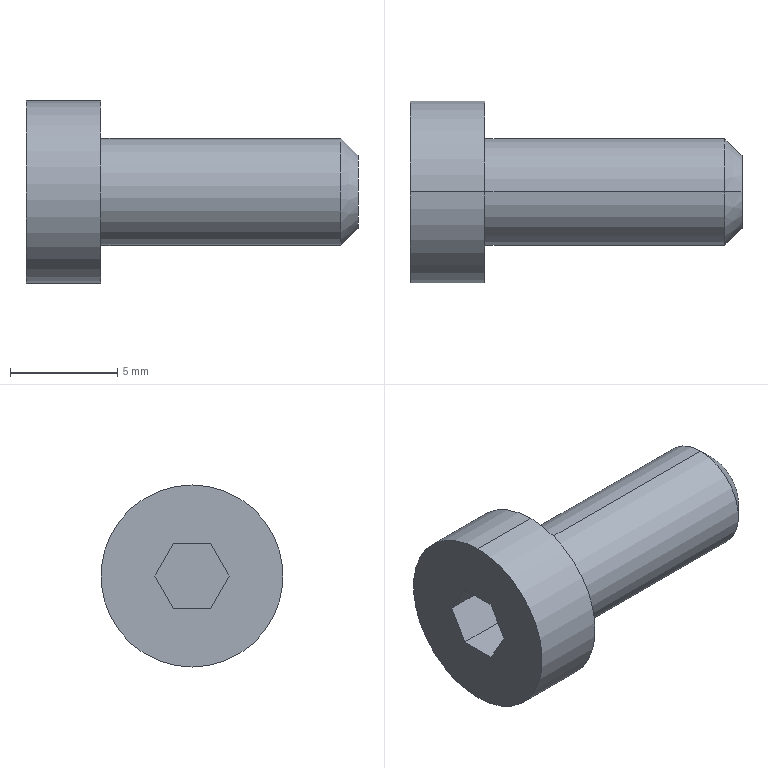Part | STEP file | CBSST5-12-10 | 1 solid | 16 faces | box 15.5 x 8.5 x 8.5 mm | volume 408.692 mm3 | plane 10 | cylinder 4 | cone 2 | commonest cylinder face diameters 5 x2 8.5 x2
STEP:
#1=CARTESIAN_POINT('',(0.,0.,4.25));
#2=VERTEX_POINT('',#1);
#3=CARTESIAN_POINT('',(0.,0.,-4.25));
#4=VERTEX_POINT('',#3);
#5=CARTESIAN_POINT('',(0.,0.,0.));
#6=DIRECTION('',(-1.,0.,0.));
#7=DIRECTION('',(0.,0.,1.));
#8=AXIS2_PLACEMENT_3D('',#5,#6,#7);
#9=CIRCLE('',#8,4.25);
#10=EDGE_CURVE('',#2,#4,#9,.T.);
#11=ORIENTED_EDGE('',*,*,#10,.T.);
#12=CARTESIAN_POINT('',(-3.5,0.,-4.25));
#13=VERTEX_POINT('',#12);
#14=CARTESIAN_POINT('',(-4.275,0.,-4.25));
#15=DIRECTION('',(-1.,0.,0.));
#16=VECTOR('',#15,1000.);
#17=LINE('',#14,#16);
#18=EDGE_CURVE('',#4,#13,#17,.T.);
#19=ORIENTED_EDGE('',*,*,#18,.T.);
#20=CARTESIAN_POINT('',(-3.5,0.,4.25));
#21=VERTEX_POINT('',#20);
#22=CARTESIAN_POINT('',(-3.5,0.,0.));
#23=DIRECTION('',(-1.,0.,0.));
#24=DIRECTION('',(0.,0.,1.));
#25=AXIS2_PLACEMENT_3D('',#22,#23,#24);
#26=CIRCLE('',#25,4.25);
#27=EDGE_CURVE('',#21,#13,#26,.T.);
#28=ORIENTED_EDGE('',*,*,#27,.F.);
#29=CARTESIAN_POINT('',(-4.275,0.,4.25));
#30=DIRECTION('',(-1.,0.,0.));
#31=VECTOR('',#30,1000.);
#32=LINE('',#29,#31);
#33=EDGE_CURVE('',#2,#21,#32,.T.);
#34=ORIENTED_EDGE('',*,*,#33,.F.);
#35=EDGE_LOOP('',(#11,#19,#28,#34));
#36=FACE_OUTER_BOUND('',#35,.T.);
#37=CARTESIAN_POINT('',(-4.275,0.,0.));
#38=DIRECTION('',(-1.,0.,0.));
#39=DIRECTION('',(0.,0.,1.));
#40=AXIS2_PLACEMENT_3D('',#37,#38,#39);
#41=CYLINDRICAL_SURFACE('',#40,4.25);
#42=ADVANCED_FACE('',(#36),#41,.T.);
#43=CARTESIAN_POINT('',(11.2,0.,2.5));
#44=VERTEX_POINT('',#43);
#45=CARTESIAN_POINT('',(11.2,0.,-2.5));
#46=VERTEX_POINT('',#45);
#47=CARTESIAN_POINT('',(11.2,0.,0.));
#48=DIRECTION('',(-1.,0.,0.));
#49=DIRECTION('',(0.,0.,1.));
#50=AXIS2_PLACEMENT_3D('',#47,#48,#49);
#51=CIRCLE('',#50,2.5);
#52=EDGE_CURVE('',#44,#46,#51,.T.);
#53=ORIENTED_EDGE('',*,*,#52,.T.);
#54=CARTESIAN_POINT('',(0.,0.,-2.5));
#55=VERTEX_POINT('',#54);
#56=CARTESIAN_POINT('',(-4.275,0.,-2.5));
#57=DIRECTION('',(-1.,0.,0.));
#58=VECTOR('',#57,1000.);
#59=LINE('',#56,#58);
#60=EDGE_CURVE('',#46,#55,#59,.T.);
#61=ORIENTED_EDGE('',*,*,#60,.T.);
#62=CARTESIAN_POINT('',(0.,0.,2.5));
#63=VERTEX_POINT('',#62);
#64=CARTESIAN_POINT('',(0.,0.,0.));
#65=DIRECTION('',(1.,0.,0.));
#66=DIRECTION('',(0.,0.,-1.));
#67=AXIS2_PLACEMENT_3D('',#64,#65,#66);
#68=CIRCLE('',#67,2.5);
#69=EDGE_CURVE('',#55,#63,#68,.T.);
#70=ORIENTED_EDGE('',*,*,#69,.T.);
#71=CARTESIAN_POINT('',(-4.275,0.,2.5));
#72=DIRECTION('',(-1.,0.,0.));
#73=VECTOR('',#72,1000.);
#74=LINE('',#71,#73);
#75=EDGE_CURVE('',#44,#63,#74,.T.);
#76=ORIENTED_EDGE('',*,*,#75,.F.);
#77=EDGE_LOOP('',(#53,#61,#70,#76));
#78=FACE_OUTER_BOUND('',#77,.T.);
#79=CARTESIAN_POINT('',(-4.275,0.,0.));
#80=DIRECTION('',(-1.,0.,0.));
#81=DIRECTION('',(0.,0.,1.));
#82=AXIS2_PLACEMENT_3D('',#79,#80,#81);
#83=CYLINDRICAL_SURFACE('',#82,2.5);
#84=ADVANCED_FACE('',(#78),#83,.T.);
#85=CARTESIAN_POINT('',(12.,0.,1.7));
#86=VERTEX_POINT('',#85);
#87=CARTESIAN_POINT('',(12.,0.,-1.7));
#88=VERTEX_POINT('',#87);
#89=CARTESIAN_POINT('',(12.,0.,0.));
#90=DIRECTION('',(-1.,0.,0.));
#91=DIRECTION('',(0.,0.,1.));
#92=AXIS2_PLACEMENT_3D('',#89,#90,#91);
#93=CIRCLE('',#92,1.7);
#94=EDGE_CURVE('',#86,#88,#93,.T.);
#95=ORIENTED_EDGE('',*,*,#94,.T.);
#96=CARTESIAN_POINT('',(11.2,0.,-2.5));
#97=DIRECTION('',(-0.7071,0.,-0.7071));
#98=VECTOR('',#97,1000.);
#99=LINE('',#96,#98);
#100=EDGE_CURVE('',#88,#46,#99,.T.);
#101=ORIENTED_EDGE('',*,*,#100,.T.);
#102=ORIENTED_EDGE('',*,*,#52,.F.);
#103=CARTESIAN_POINT('',(11.2,0.,2.5));
#104=DIRECTION('',(-0.7071,0.,0.7071));
#105=VECTOR('',#104,1000.);
#106=LINE('',#103,#105);
#107=EDGE_CURVE('',#86,#44,#106,.T.);
#108=ORIENTED_EDGE('',*,*,#107,.F.);
#109=EDGE_LOOP('',(#95,#101,#102,#108));
#110=FACE_OUTER_BOUND('',#109,.T.);
#111=CARTESIAN_POINT('',(11.2,0.,0.));
#112=DIRECTION('',(-1.,0.,0.));
#113=DIRECTION('',(0.,0.,1.));
#114=AXIS2_PLACEMENT_3D('',#111,#112,#113);
#115=CONICAL_SURFACE('',#114,2.5,0.7854);
#116=ADVANCED_FACE('',(#110),#115,.T.);
#117=CARTESIAN_POINT('',(-3.5,0.866,1.5));
#118=VERTEX_POINT('',#117);
#119=CARTESIAN_POINT('',(-3.5,1.732,0.));
#120=VERTEX_POINT('',#119);
#121=CARTESIAN_POINT('',(-3.5,0.866,1.5));
#122=DIRECTION('',(0.,0.5,-0.866));
#123=VECTOR('',#122,1000.);
#124=LINE('',#121,#123);
#125=EDGE_CURVE('',#118,#120,#124,.T.);
#126=ORIENTED_EDGE('',*,*,#125,.F.);
#127=CARTESIAN_POINT('',(-3.5,-0.866,1.5));
#128=VERTEX_POINT('',#127);
#129=CARTESIAN_POINT('',(-3.5,-0.866,1.5));
#130=DIRECTION('',(0.,1.,0.));
#131=VECTOR('',#130,1000.);
#132=LINE('',#129,#131);
#133=EDGE_CURVE('',#128,#118,#132,.T.);
#134=ORIENTED_EDGE('',*,*,#133,.F.);
#135=CARTESIAN_POINT('',(-3.5,-1.732,0.));
#136=VERTEX_POINT('',#135);
#137=CARTESIAN_POINT('',(-3.5,-1.732,0.));
#138=DIRECTION('',(0.,0.5,0.866));
#139=VECTOR('',#138,1000.);
#140=LINE('',#137,#139);
#141=EDGE_CURVE('',#136,#128,#140,.T.);
#142=ORIENTED_EDGE('',*,*,#141,.F.);
#143=CARTESIAN_POINT('',(-3.5,-0.866,-1.5));
#144=VERTEX_POINT('',#143);
#145=CARTESIAN_POINT('',(-3.5,-0.866,-1.5));
#146=DIRECTION('',(0.,-0.5,0.866));
#147=VECTOR('',#146,1000.);
#148=LINE('',#145,#147);
#149=EDGE_CURVE('',#144,#136,#148,.T.);
#150=ORIENTED_EDGE('',*,*,#149,.F.);
#151=CARTESIAN_POINT('',(-3.5,0.866,-1.5));
#152=VERTEX_POINT('',#151);
#153=CARTESIAN_POINT('',(-3.5,0.866,-1.5));
#154=DIRECTION('',(0.,-1.,0.));
#155=VECTOR('',#154,1000.);
#156=LINE('',#153,#155);
#157=EDGE_CURVE('',#152,#144,#156,.T.);
#158=ORIENTED_EDGE('',*,*,#157,.F.);
#159=CARTESIAN_POINT('',(-3.5,1.732,0.));
#160=DIRECTION('',(0.,-0.5,-0.866));
#161=VECTOR('',#160,1000.);
#162=LINE('',#159,#161);
#163=EDGE_CURVE('',#120,#152,#162,.T.);
#164=ORIENTED_EDGE('',*,*,#163,.F.);
#165=EDGE_LOOP('',(#126,#134,#142,#150,#158,#164));
#166=FACE_BOUND('',#165,.T.);
#167=ORIENTED_EDGE('',*,*,#27,.T.);
#168=CARTESIAN_POINT('',(-3.5,0.,0.));
#169=DIRECTION('',(-1.,0.,0.));
#170=DIRECTION('',(0.,0.,1.));
#171=AXIS2_PLACEMENT_3D('',#168,#169,#170);
#172=CIRCLE('',#171,4.25);
#173=EDGE_CURVE('',#13,#21,#172,.T.);
#174=ORIENTED_EDGE('',*,*,#173,.T.);
#175=EDGE_LOOP('',(#167,#174));
#176=FACE_OUTER_BOUND('',#175,.T.);
#177=CARTESIAN_POINT('',(-3.5,-4.25,0.));
#178=DIRECTION('',(-1.,0.,0.));
#179=DIRECTION('',(0.,0.,1.));
#180=AXIS2_PLACEMENT_3D('',#177,#178,#179);
#181=PLANE('',#180);
#182=ADVANCED_FACE('',(#166,#176),#181,.T.);
#183=ORIENTED_EDGE('',*,*,#94,.F.);
#184=CARTESIAN_POINT('',(12.,0.,0.));
#185=DIRECTION('',(-1.,0.,0.));
#186=DIRECTION('',(0.,0.,1.));
#187=AXIS2_PLACEMENT_3D('',#184,#185,#186);
#188=CIRCLE('',#187,1.7);
#189=EDGE_CURVE('',#88,#86,#188,.T.);
#190=ORIENTED_EDGE('',*,*,#189,.F.);
#191=EDGE_LOOP('',(#183,#190));
#192=FACE_OUTER_BOUND('',#191,.T.);
#193=CARTESIAN_POINT('',(12.,0.,0.));
#194=DIRECTION('',(1.,0.,0.));
#195=DIRECTION('',(0.,0.,-1.));
#196=AXIS2_PLACEMENT_3D('',#193,#194,#195);
#197=PLANE('',#196);
#198=ADVANCED_FACE('',(#192),#197,.T.);
#199=ORIENTED_EDGE('',*,*,#100,.F.);
#200=ORIENTED_EDGE('',*,*,#189,.T.);
#201=ORIENTED_EDGE('',*,*,#107,.T.);
#202=CARTESIAN_POINT('',(11.2,0.,0.));
#203=DIRECTION('',(-1.,0.,0.));
#204=DIRECTION('',(0.,0.,1.));
#205=AXIS2_PLACEMENT_3D('',#202,#203,#204);
#206=CIRCLE('',#205,2.5);
#207=EDGE_CURVE('',#46,#44,#206,.T.);
#208=ORIENTED_EDGE('',*,*,#207,.F.);
#209=EDGE_LOOP('',(#199,#200,#201,#208));
#210=FACE_OUTER_BOUND('',#209,.T.);
#211=CARTESIAN_POINT('',(11.2,0.,0.));
#212=DIRECTION('',(-1.,0.,0.));
#213=DIRECTION('',(0.,0.,1.));
#214=AXIS2_PLACEMENT_3D('',#211,#212,#213);
#215=CONICAL_SURFACE('',#214,2.5,0.7854);
#216=ADVANCED_FACE('',(#210),#215,.T.);
#217=ORIENTED_EDGE('',*,*,#60,.F.);
#218=ORIENTED_EDGE('',*,*,#207,.T.);
#219=ORIENTED_EDGE('',*,*,#75,.T.);
#220=CARTESIAN_POINT('',(0.,0.,0.));
#221=DIRECTION('',(1.,0.,0.));
#222=DIRECTION('',(0.,0.,-1.));
#223=AXIS2_PLACEMENT_3D('',#220,#221,#222);
#224=CIRCLE('',#223,2.5);
#225=EDGE_CURVE('',#63,#55,#224,.T.);
#226=ORIENTED_EDGE('',*,*,#225,.T.);
#227=EDGE_LOOP('',(#217,#218,#219,#226));
#228=FACE_OUTER_BOUND('',#227,.T.);
#229=CARTESIAN_POINT('',(-4.275,0.,0.));
#230=DIRECTION('',(-1.,0.,0.));
#231=DIRECTION('',(0.,0.,1.));
#232=AXIS2_PLACEMENT_3D('',#229,#230,#231);
#233=CYLINDRICAL_SURFACE('',#232,2.5);
#234=ADVANCED_FACE('',(#228),#233,.T.);
#235=ORIENTED_EDGE('',*,*,#10,.F.);
#236=CARTESIAN_POINT('',(0.,0.,0.));
#237=DIRECTION('',(-1.,0.,0.));
#238=DIRECTION('',(0.,0.,1.));
#239=AXIS2_PLACEMENT_3D('',#236,#237,#238);
#240=CIRCLE('',#239,4.25);
#241=EDGE_CURVE('',#4,#2,#240,.T.);
#242=ORIENTED_EDGE('',*,*,#241,.F.);
#243=EDGE_LOOP('',(#235,#242));
#244=FACE_OUTER_BOUND('',#243,.T.);
#245=ORIENTED_EDGE('',*,*,#225,.F.);
#246=ORIENTED_EDGE('',*,*,#69,.F.);
#247=EDGE_LOOP('',(#245,#246));
#248=FACE_BOUND('',#247,.T.);
#249=CARTESIAN_POINT('',(0.,-2.7,0.));
#250=DIRECTION('',(1.,0.,0.));
#251=DIRECTION('',(0.,0.,-1.));
#252=AXIS2_PLACEMENT_3D('',#249,#250,#251);
#253=PLANE('',#252);
#254=ADVANCED_FACE('',(#244,#248),#253,.T.);
#255=ORIENTED_EDGE('',*,*,#18,.F.);
#256=ORIENTED_EDGE('',*,*,#241,.T.);
#257=ORIENTED_EDGE('',*,*,#33,.T.);
#258=ORIENTED_EDGE('',*,*,#173,.F.);
#259=EDGE_LOOP('',(#255,#256,#257,#258));
#260=FACE_OUTER_BOUND('',#259,.T.);
#261=CARTESIAN_POINT('',(-4.275,0.,0.));
#262=DIRECTION('',(-1.,0.,0.));
#263=DIRECTION('',(0.,0.,1.));
#264=AXIS2_PLACEMENT_3D('',#261,#262,#263);
#265=CYLINDRICAL_SURFACE('',#264,4.25);
#266=ADVANCED_FACE('',(#260),#265,.T.);
#267=ORIENTED_EDGE('',*,*,#125,.T.);
#268=CARTESIAN_POINT('',(-0.8,1.732,0.));
#269=VERTEX_POINT('',#268);
#270=CARTESIAN_POINT('',(-0.8,1.732,0.));
#271=DIRECTION('',(-1.,0.,0.));
#272=VECTOR('',#271,1000.);
#273=LINE('',#270,#272);
#274=EDGE_CURVE('',#269,#120,#273,.T.);
#275=ORIENTED_EDGE('',*,*,#274,.F.);
#276=CARTESIAN_POINT('',(-0.8,0.866,1.5));
#277=VERTEX_POINT('',#276);
#278=CARTESIAN_POINT('',(-0.8,0.866,1.5));
#279=DIRECTION('',(0.,0.5,-0.866));
#280=VECTOR('',#279,1000.);
#281=LINE('',#278,#280);
#282=EDGE_CURVE('',#277,#269,#281,.T.);
#283=ORIENTED_EDGE('',*,*,#282,.F.);
#284=CARTESIAN_POINT('',(-0.8,0.866,1.5));
#285=DIRECTION('',(-1.,0.,0.));
#286=VECTOR('',#285,1000.);
#287=LINE('',#284,#286);
#288=EDGE_CURVE('',#277,#118,#287,.T.);
#289=ORIENTED_EDGE('',*,*,#288,.T.);
#290=EDGE_LOOP('',(#267,#275,#283,#289));
#291=FACE_OUTER_BOUND('',#290,.T.);
#292=CARTESIAN_POINT('',(-0.8,0.866,1.5));
#293=DIRECTION('',(0.,0.866,0.5));
#294=DIRECTION('',(0.,-0.5,0.866));
#295=AXIS2_PLACEMENT_3D('',#292,#293,#294);
#296=PLANE('',#295);
#297=ADVANCED_FACE('',(#291),#296,.F.);
#298=ORIENTED_EDGE('',*,*,#133,.T.);
#299=ORIENTED_EDGE('',*,*,#288,.F.);
#300=CARTESIAN_POINT('',(-0.8,-0.866,1.5));
#301=VERTEX_POINT('',#300);
#302=CARTESIAN_POINT('',(-0.8,-0.866,1.5));
#303=DIRECTION('',(0.,1.,0.));
#304=VECTOR('',#303,1000.);
#305=LINE('',#302,#304);
#306=EDGE_CURVE('',#301,#277,#305,.T.);
#307=ORIENTED_EDGE('',*,*,#306,.F.);
#308=CARTESIAN_POINT('',(-0.8,-0.866,1.5));
#309=DIRECTION('',(-1.,0.,0.));
#310=VECTOR('',#309,1000.);
#311=LINE('',#308,#310);
#312=EDGE_CURVE('',#301,#128,#311,.T.);
#313=ORIENTED_EDGE('',*,*,#312,.T.);
#314=EDGE_LOOP('',(#298,#299,#307,#313));
#315=FACE_OUTER_BOUND('',#314,.T.);
#316=CARTESIAN_POINT('',(-0.8,-0.866,1.5));
#317=DIRECTION('',(0.,0.,1.));
#318=DIRECTION('',(0.,-1.,0.));
#319=AXIS2_PLACEMENT_3D('',#316,#317,#318);
#320=PLANE('',#319);
#321=ADVANCED_FACE('',(#315),#320,.F.);
#322=ORIENTED_EDGE('',*,*,#141,.T.);
#323=ORIENTED_EDGE('',*,*,#312,.F.);
#324=CARTESIAN_POINT('',(-0.8,-1.732,0.));
#325=VERTEX_POINT('',#324);
#326=CARTESIAN_POINT('',(-0.8,-1.732,0.));
#327=DIRECTION('',(0.,0.5,0.866));
#328=VECTOR('',#327,1000.);
#329=LINE('',#326,#328);
#330=EDGE_CURVE('',#325,#301,#329,.T.);
#331=ORIENTED_EDGE('',*,*,#330,.F.);
#332=CARTESIAN_POINT('',(-0.8,-1.732,0.));
#333=DIRECTION('',(-1.,0.,0.));
#334=VECTOR('',#333,1000.);
#335=LINE('',#332,#334);
#336=EDGE_CURVE('',#325,#136,#335,.T.);
#337=ORIENTED_EDGE('',*,*,#336,.T.);
#338=EDGE_LOOP('',(#322,#323,#331,#337));
#339=FACE_OUTER_BOUND('',#338,.T.);
#340=CARTESIAN_POINT('',(-0.8,-1.732,0.));
#341=DIRECTION('',(0.,-0.866,0.5));
#342=DIRECTION('',(0.,-0.5,-0.866));
#343=AXIS2_PLACEMENT_3D('',#340,#341,#342);
#344=PLANE('',#343);
#345=ADVANCED_FACE('',(#339),#344,.F.);
#346=ORIENTED_EDGE('',*,*,#149,.T.);
#347=ORIENTED_EDGE('',*,*,#336,.F.);
#348=CARTESIAN_POINT('',(-0.8,-0.866,-1.5));
#349=VERTEX_POINT('',#348);
#350=CARTESIAN_POINT('',(-0.8,-0.866,-1.5));
#351=DIRECTION('',(0.,-0.5,0.866));
#352=VECTOR('',#351,1000.);
#353=LINE('',#350,#352);
#354=EDGE_CURVE('',#349,#325,#353,.T.);
#355=ORIENTED_EDGE('',*,*,#354,.F.);
#356=CARTESIAN_POINT('',(-0.8,-0.866,-1.5));
#357=DIRECTION('',(-1.,0.,0.));
#358=VECTOR('',#357,1000.);
#359=LINE('',#356,#358);
#360=EDGE_CURVE('',#349,#144,#359,.T.);
#361=ORIENTED_EDGE('',*,*,#360,.T.);
#362=EDGE_LOOP('',(#346,#347,#355,#361));
#363=FACE_OUTER_BOUND('',#362,.T.);
#364=CARTESIAN_POINT('',(-0.8,-0.866,-1.5));
#365=DIRECTION('',(0.,-0.866,-0.5));
#366=DIRECTION('',(0.,0.5,-0.866));
#367=AXIS2_PLACEMENT_3D('',#364,#365,#366);
#368=PLANE('',#367);
#369=ADVANCED_FACE('',(#363),#368,.F.);
#370=ORIENTED_EDGE('',*,*,#157,.T.);
#371=ORIENTED_EDGE('',*,*,#360,.F.);
#372=CARTESIAN_POINT('',(-0.8,0.866,-1.5));
#373=VERTEX_POINT('',#372);
#374=CARTESIAN_POINT('',(-0.8,0.866,-1.5));
#375=DIRECTION('',(0.,-1.,0.));
#376=VECTOR('',#375,1000.);
#377=LINE('',#374,#376);
#378=EDGE_CURVE('',#373,#349,#377,.T.);
#379=ORIENTED_EDGE('',*,*,#378,.F.);
#380=CARTESIAN_POINT('',(-0.8,0.866,-1.5));
#381=DIRECTION('',(-1.,0.,0.));
#382=VECTOR('',#381,1000.);
#383=LINE('',#380,#382);
#384=EDGE_CURVE('',#373,#152,#383,.T.);
#385=ORIENTED_EDGE('',*,*,#384,.T.);
#386=EDGE_LOOP('',(#370,#371,#379,#385));
#387=FACE_OUTER_BOUND('',#386,.T.);
#388=CARTESIAN_POINT('',(-0.8,0.866,-1.5));
#389=DIRECTION('',(0.,0.,-1.));
#390=DIRECTION('',(-1.,0.,0.));
#391=AXIS2_PLACEMENT_3D('',#388,#389,#390);
#392=PLANE('',#391);
#393=ADVANCED_FACE('',(#387),#392,.F.);
#394=ORIENTED_EDGE('',*,*,#163,.T.);
#395=ORIENTED_EDGE('',*,*,#384,.F.);
#396=CARTESIAN_POINT('',(-0.8,1.732,0.));
#397=DIRECTION('',(0.,-0.5,-0.866));
#398=VECTOR('',#397,1000.);
#399=LINE('',#396,#398);
#400=EDGE_CURVE('',#269,#373,#399,.T.);
#401=ORIENTED_EDGE('',*,*,#400,.F.);
#402=ORIENTED_EDGE('',*,*,#274,.T.);
#403=EDGE_LOOP('',(#394,#395,#401,#402));
#404=FACE_OUTER_BOUND('',#403,.T.);
#405=CARTESIAN_POINT('',(-0.8,1.732,0.));
#406=DIRECTION('',(0.,0.866,-0.5));
#407=DIRECTION('',(0.,0.5,0.866));
#408=AXIS2_PLACEMENT_3D('',#405,#406,#407);
#409=PLANE('',#408);
#410=ADVANCED_FACE('',(#404),#409,.F.);
#411=ORIENTED_EDGE('',*,*,#282,.T.);
#412=ORIENTED_EDGE('',*,*,#400,.T.);
#413=ORIENTED_EDGE('',*,*,#378,.T.);
#414=ORIENTED_EDGE('',*,*,#354,.T.);
#415=ORIENTED_EDGE('',*,*,#330,.T.);
#416=ORIENTED_EDGE('',*,*,#306,.T.);
#417=EDGE_LOOP('',(#411,#412,#413,#414,#415,#416));
#418=FACE_OUTER_BOUND('',#417,.T.);
#419=CARTESIAN_POINT('',(-0.8,0.,0.));
#420=DIRECTION('',(-1.,0.,0.));
#421=DIRECTION('',(0.,0.,1.));
#422=AXIS2_PLACEMENT_3D('',#419,#420,#421);
#423=PLANE('',#422);
#424=ADVANCED_FACE('',(#418),#423,.T.);
#425=CLOSED_SHELL('',(#42,#84,#116,#182,#198,#216,#234,#254,#266,#297,#321,#345,#369,#393,#410,#424));
#426=MANIFOLD_SOLID_BREP('',#425);
#427=CARTESIAN_POINT('',(0.,0.,0.));
#428=DIRECTION('',(0.,0.,1.));
#429=DIRECTION('',(1.,0.,0.));
#430=AXIS2_PLACEMENT_3D('',#427,#428,#429);
#431=(LENGTH_UNIT()NAMED_UNIT(*)SI_UNIT(.MILLI.,.METRE.));
#432=UNCERTAINTY_MEASURE_WITH_UNIT(LENGTH_MEASURE(0.00001),#431,'','');
#433=(NAMED_UNIT(*)PLANE_ANGLE_UNIT()SI_UNIT($,.RADIAN.));
#434=(NAMED_UNIT(*)SI_UNIT($,.STERADIAN.)SOLID_ANGLE_UNIT());
#435=(GEOMETRIC_REPRESENTATION_CONTEXT(3)GLOBAL_UNCERTAINTY_ASSIGNED_CONTEXT((#432))GLOBAL_UNIT_ASSIGNED_CONTEXT((#431,#433,#434))REPRESENTATION_CONTEXT('',''));
#436=ADVANCED_BREP_SHAPE_REPRESENTATION('',(#426,#430),#435);